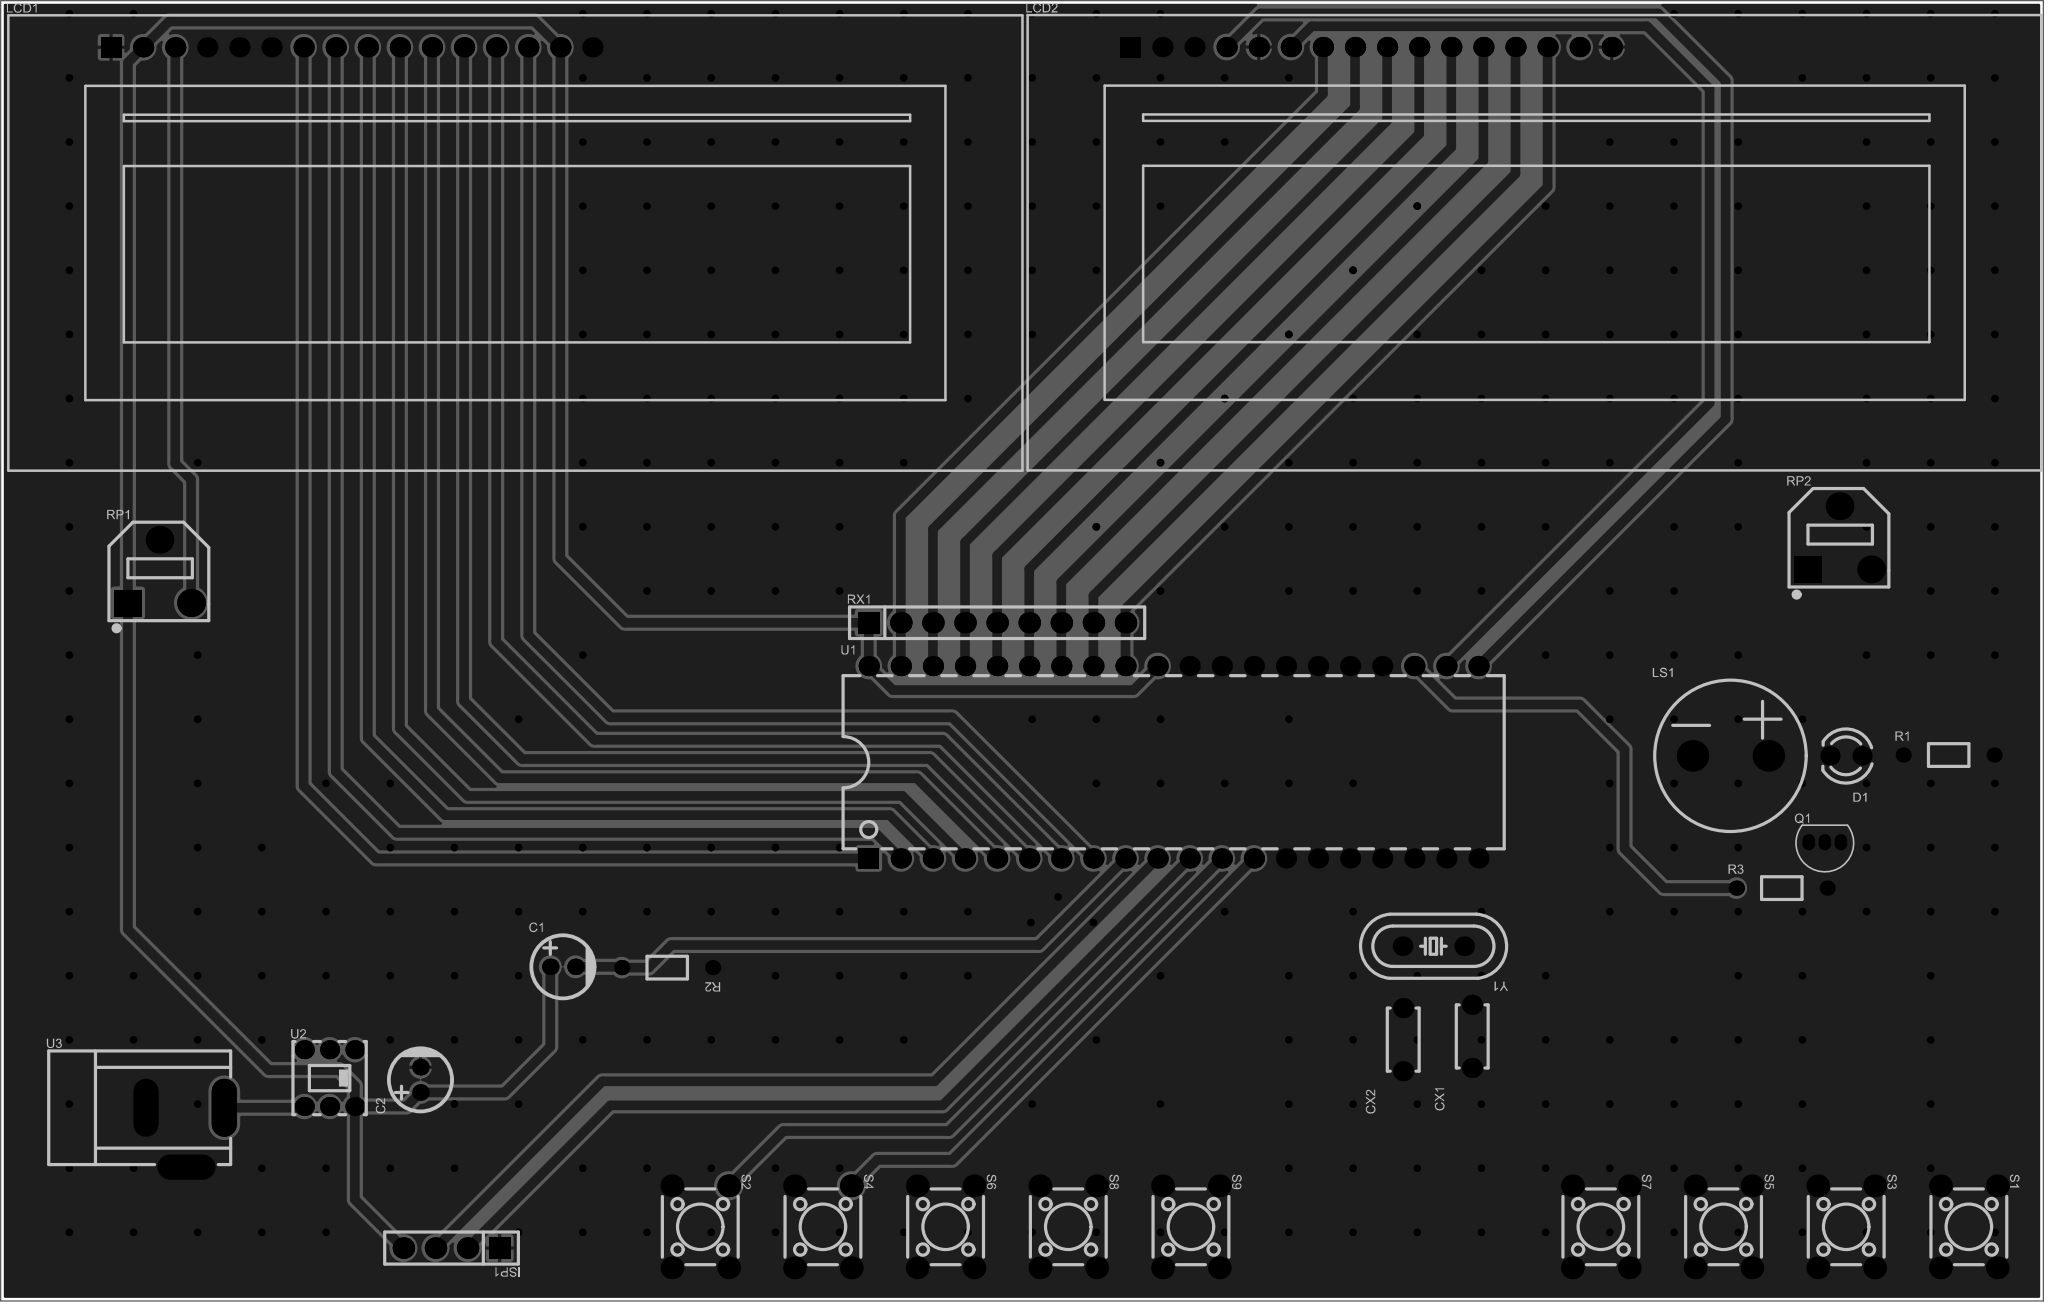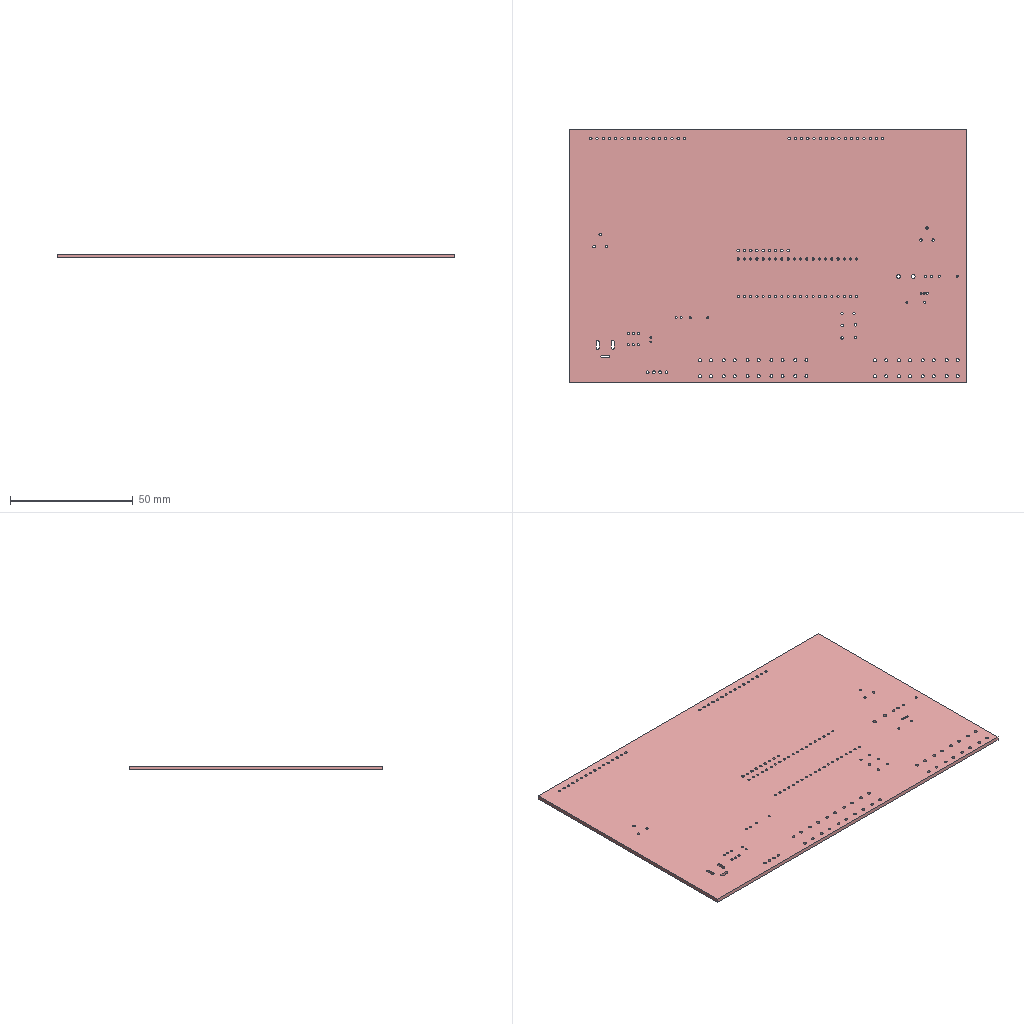Circuit board layout | Altium Designer | box 161.7 x 103 x 1.6 mm
Layer stack:
# Altium Designer layer stack of  (unit mm; dielectric type: 0 none, 1 core, 2 prepreg, 3 surface material)
index,name,kind,layer,copper_thickness_mm,dielectric_type,dielectric_thickness_mm,dielectric_material,dielectric_constant
0,Top Paste Mask Layer,other,,,,,,
1,Top Silkscreen Layer,other,,,,,,
2,Top Solder Mask Layer,dielectric,,,3,0.01,,3.3
3,Top Layer,copper,Top Layer,0.035,,,,
4,Dielectric1,dielectric,,,3,1.51,FR4,4.5
5,Bottom Layer,copper,Bottom Layer,0.035,,,,
6,Bottom Solder Mask Layer,dielectric,,,3,0.01,,3.3
7,Bottom Silkscreen Layer,other,,,,,,
8,Bottom Paste Mask Layer,other,,,,,,
# drill layer pairs: low layer,high layer
drill_pair,Top Layer,Bottom Layer
Part placement:
Designator,Comment,Layer,Footprint,Center-X(mm),Center-Y(mm),Rotation
C1,Cap Pol2,TopLayer,CAP-TH_BD5.0-P2.00-D0.8-FD-10UF50VC110GL,129.337,111.303,0
C2,1000UF,TopLayer,CAP-TH_BD5.0-P2.00-D0.8-FD-10UF50VC110GL,118.063,102.35,90
D1,LED1,TopLayer,LED_TH-3mm,230.886,128.016,180
ISP1,Header 4,TopLayer,HDR-TH_4P-P2.54-V-F,120.523,89.027,180
LCD1,1602,TopLayer,LCD1602,112.626,184.136,0
LCD2,1602,TopLayer,LCD1602,193.298,184.156,0
LS1,Bell,TopLayer,BUZ-TH_BD12.0-P6.00-D0.9-RD,221.742,128.016,0
Q1,2N3906,TopLayer,TO-92-3_L4.6-W3.6-P1.27-L_1,229.212,121.173,0
R1,Res2,TopLayer,Res_1/8W,239.014,128.079,0
R2,Res2,TopLayer,Res_1/8W,137.592,111.24,180
R3,Res2,TopLayer,Res_1/8W,225.806,117.538,0
RP1,RPot,TopLayer,RES-ADJ-SMD_RM065-V1,97.409,142.621,0
RP2,RPot,TopLayer,RES-ADJ-SMD_RM065-V1,230.378,145.288,0
RX1,Header 9,TopLayer,HDR-TH_9P-P2.54-V-F-1,163.703,138.557,0
S1,SW-PB,TopLayer,SW-TH_4P-L6.0-W6.0-P4.50-LS6.5,240.61,90.71,270
S2,SW-PB,TopLayer,SW-TH_4P-L6.0-W6.0-P4.50-LS6.5,140.208,90.71,270
S3,SW-PB,TopLayer,SW-TH_4P-L6.0-W6.0-P4.50-LS6.5,230.902,90.71,270
S4,SW-PB,TopLayer,SW-TH_4P-L6.0-W6.0-P4.50-LS6.5,149.917,90.71,270
S5,SW-PB,TopLayer,SW-TH_4P-L6.0-W6.0-P4.50-LS6.5,221.193,90.71,270
S6,SW-PB,TopLayer,SW-TH_4P-L6.0-W6.0-P4.50-LS6.5,159.625,90.71,270
S7,SW-PB,TopLayer,SW-TH_4P-L6.0-W6.0-P4.50-LS6.5,211.484,90.71,270
S8,SW-PB,TopLayer,SW-TH_4P-L6.0-W6.0-P4.50-LS6.5,169.334,90.71,270
S9,SW-PB,TopLayer,SW-TH_4P-L6.0-W6.0-P4.50-LS6.5,179.043,90.71,270
U1,STC89C52,TopLayer,DIP-40_L52.0-W13.7-P2.54-LS15.2-BL,177.673,127.508,0
U2,SWITCH,TopLayer,SW-TH_6P-L5.8-W5.8-P2.00-LS4.5-BL,110.871,102.489,0
U3,POW,TopLayer,DC-IN-TH_DC005,99.441,97.79,0
Y1,XTAL,TopLayer,HC-49S_L11.5-W5.0-P4.88,198.23,112.935,180
CX1,Cap,TopLayer,CAP-TH_L5.0-W2.5-P5.00-D1.0,201.295,105.791,90
CX2,Cap,TopLayer,CAP-TH_L5.0-W2.5-P5.00-D1.0,195.834,105.537,90
Pad and via stacks:
# Altium Designer via and pad stacks of  (unit mm). Each distinct definition once, with the count of objects using it.
# via: kind,start_layer,end_layer,hole_mm,diameter_mm,mode(0 simple;1 top-mid-bottom;2 full stack),diameter_per_layer,count,example_net
# pad: kind,layer,hole_mm,hole_type(0 round;1 square;2 slot),plating,top_size,top_shape(1 round;2 rect;3 octagon;9 rounded rect),mid_size,bottom_size,mode,footprint,size_per_layer,count,example
pad,Multi-Layer,0.8,0,plated,1.3x1.3,1,1.3x1.3,1.3x1.3,0,CAP-TH_BD5.0-P2.00-D0.8-FD-10UF50VC110GL,,4,C1.2
pad,Multi-Layer,0.9144,0,plated,1.524x1.524,1,1.524x1.524,1.524x1.524,0,LED_TH-3mm,,2,D1.1
pad,Multi-Layer,1.1,0,plated,1.7x1.7,2,1.7x1.7,1.7x1.7,0,HDR-TH_4P-P2.54-V-F,,1,ISP1.1
pad,Multi-Layer,1.1,0,plated,1.7x1.7,1,1.7x1.7,1.7x1.7,0,HDR-TH_4P-P2.54-V-F,,3,ISP1.2
pad,Multi-Layer,1,0,plated,1.6x1.6,1,1.6x1.6,1.6x1.6,0,LCD1602,,30,LCD1.16
pad,Multi-Layer,1,0,plated,1.6x1.6,2,1.6x1.6,1.6x1.6,0,LCD1602,,2,LCD1.1
pad,Multi-Layer,1.5,0,plated,2.5x2.5,1,2.5x2.5,2.5x2.5,0,BUZ-TH_BD12.0-P6.00-D0.9-RD,,2,LS1.1
pad,Multi-Layer,0.8,2,plated,1x1.3,1,1x1.3,1x1.3,0,TO-92-3_L4.6-W3.6-P1.27-L_1,,3,Q1.1
pad,Multi-Layer,0.8001,0,plated,1.199x1.199,1,1.199x1.199,1.199x1.199,0,Res_1/8W,,6,R1.1
pad,Multi-Layer,1,0,plated,2.2x2.1,2,2.2x2.1,2.2x2.1,0,RES-ADJ-SMD_RM065-V1,,2,RP1.1
pad,Multi-Layer,1,0,plated,2.2x2.2,1,2.2x2.2,2.2x2.2,0,RES-ADJ-SMD_RM065-V1,,4,RP1.3
pad,Multi-Layer,1.1,0,plated,1.7x1.7,2,1.7x1.7,1.7x1.7,0,HDR-TH_9P-P2.54-V-F-1,,1,RX1.1
pad,Multi-Layer,1.1,0,plated,1.7x1.7,1,1.7x1.7,1.7x1.7,0,HDR-TH_9P-P2.54-V-F-1,,8,RX1.2
pad,Multi-Layer,1.2,0,plated,1.8x1.8,1,1.8x1.8,1.8x1.8,0,SW-TH_4P-L6.0-W6.0-P4.50-LS6.5,,36,S1.1
pad,Multi-Layer,0.889,0,plated,1.6x1.6,1,1.6x1.6,1.6x1.6,0,DIP-40_L52.0-W13.7-P2.54-LS15.2-BL,,39,U1.31
pad,Multi-Layer,0.889,0,plated,1.6x1.6,2,1.6x1.6,1.6x1.6,0,DIP-40_L52.0-W13.7-P2.54-LS15.2-BL,,1,U1.1
pad,Multi-Layer,0.9,0,plated,1.5x1.5,1,1.5x1.5,1.5x1.5,0,SW-TH_6P-L5.8-W5.8-P2.00-LS4.5-BL,,6,U2.4
pad,Multi-Layer,1.2,2,plated,2x4.6,1,2x4.6,2x4.6,0,DC-IN-TH_DC005,,2,U3.1
pad,Multi-Layer,1.2,2,plated,4.6x2,1,4.6x2,4.6x2,0,DC-IN-TH_DC005,,1,U3.3
pad,Multi-Layer,0.9,0,plated,1.56x1.56,1,1.56x1.56,1.56x1.56,0,HC-49S_L11.5-W5.0-P4.88,,2,Y1.1
pad,Multi-Layer,1,0,plated,1.6x1.6,1,1.6x1.6,1.6x1.6,0,CAP-TH_L5.0-W2.5-P5.00-D1.0,,4,CX1.1
via,Top Layer,Bottom Layer,0.3048,0.61,0,,372,TXD
Copper pours:
name,layer,net,type(0 solid;1 hatched;2 none)
Top Layer-GND,Top Layer,GND,0
Bottom Layer-GND,Bottom Layer,GND,0
Design rules, without the lines most boards share:
# Altium Designer design rules of  (exported by Altium Designer, unit mm)
# columns: name | kind | enabled | priority | scope1 | scope2 | descriptor | typed fields (field=value)
creepage | 65 | enabled | 1 | All | All | Creepage Distance Constraint =(0mil) (All),(All) |
copperRegion | 20 | enabled | 1 | (InNet('GND')) | All | Polygon Connect Rule(Relief Connect )(Conductor Width=10mil) (Relief Angle=90 Angle) (Entries=4) (Air Gap Width=10mil) ((InNet('GND'))),(All) | connect_style(0=relief,1=direct,2=none)=0 relief_conductor_width=0.254 relief_entries=4